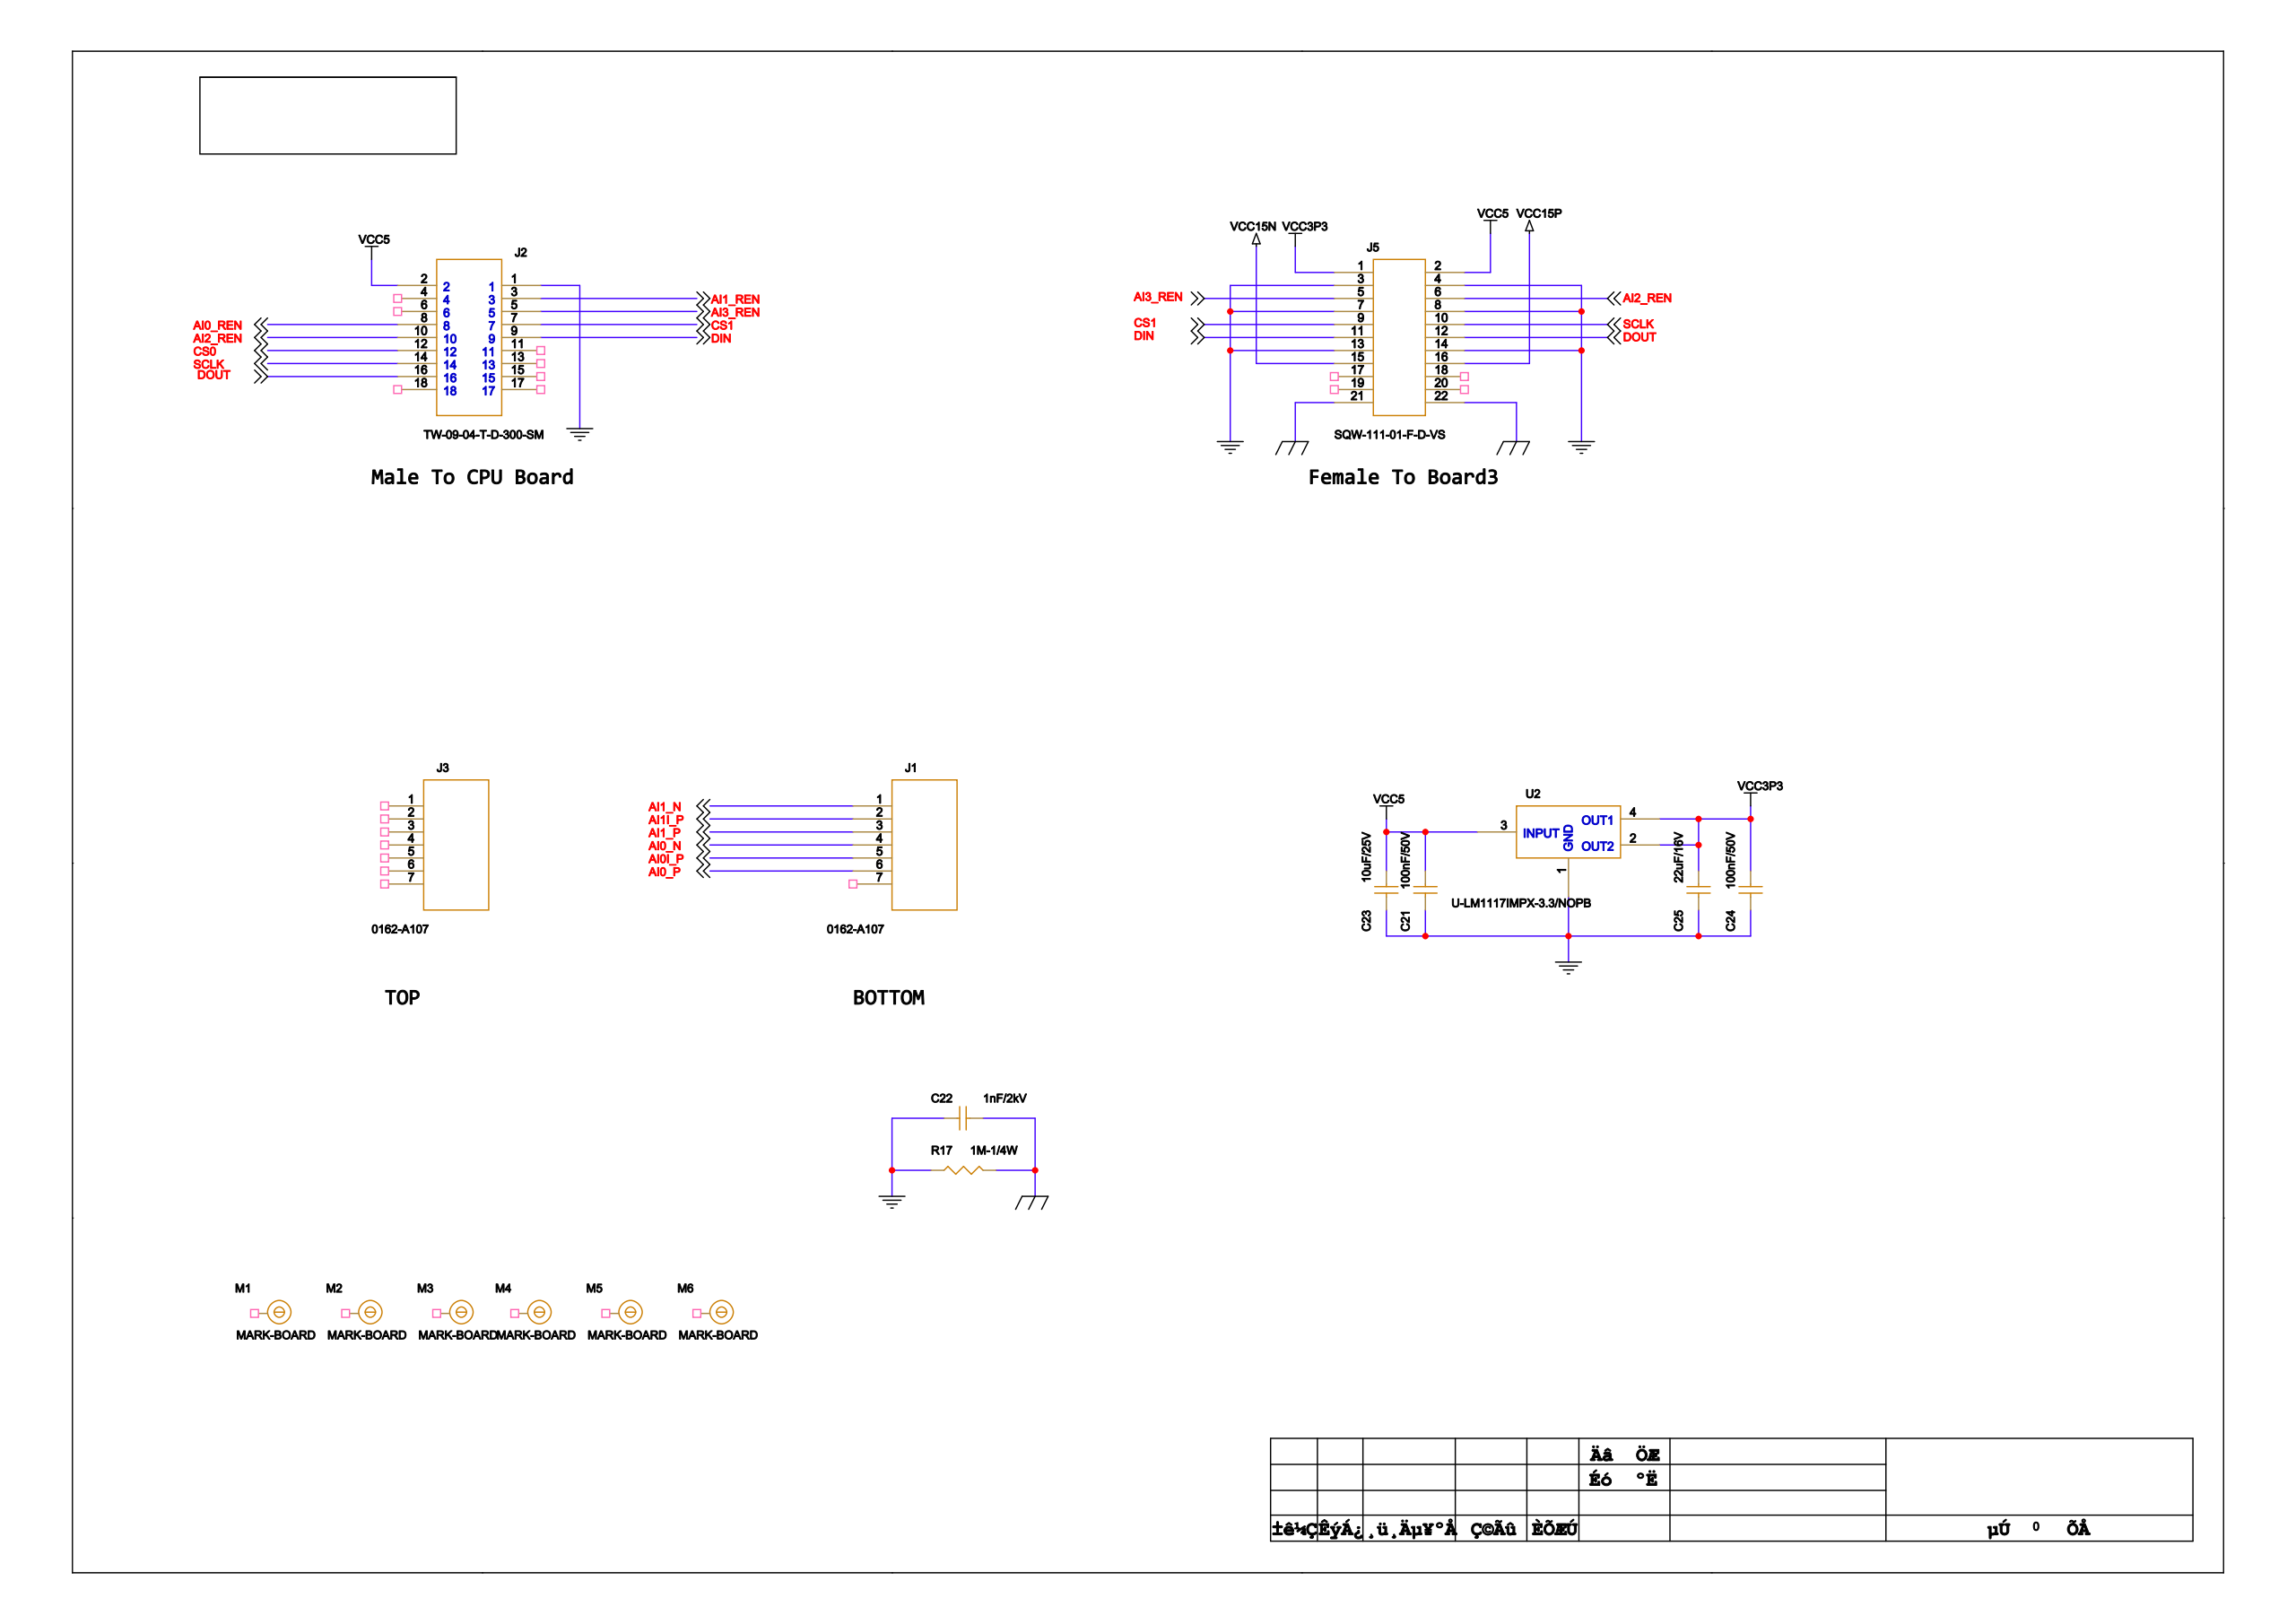Circuit board | Cadence Allegro | 65 parts | 41 nets | one sheet of the schematic
Parts on this sheet (reference | value | footprint):
C21 | 100nF/50V | C0603
C22 | 1nF/2kV | C1206
C23 | 10uF/25V | C0805
C24 | 100nF/50V | C0603
C25 | 22uF/16V | C1210
J1 | 0162-A107 | CON7-0162-A107
J2 | TW-09-04-T-D-300-SM | CON18-TW-09
J5 | SQW-111-01-F-D-VS | CON22-SQW-111
R17 | 1M-1/4W | R1210
U2 | U-LM1117IMPX-3.3/NOPB | SOT223
Nets of these parts (net: part-pin ...):
AI0_N: J1-4
AI0_REN: J2-8
AI1_N: J1-1
AI1_REN: J2-3
GND: C21-2 C22-1 C23-2 C24-2 C25-2 J2-1 J5-3 J5-4 J5-7 J5-8 J5-13 J5-14 R17-1 U2-1
VCC15P: J5-16
VCC15N: J5-15
VCC5: C21-1 C23-1 J2-2 J5-2 U2-3
VCC3P3: C24-1 C25-1 J5-1 U2-2 U2-4
AI1_P: J1-3
GND_EARTH: C22-2 J5-21 J5-22 R17-2
AI0_P: J1-6
AI1I_P: J1-2
AI0I_P: J1-5
AI2_REN: J2-10 J5-6
CS0: J2-12
SCLK: J2-14 J5-10
DOUT: J2-16 J5-12
AI3_REN: J2-5 J5-5
CS1: J2-7 J5-9
DIN: J2-9 J5-11